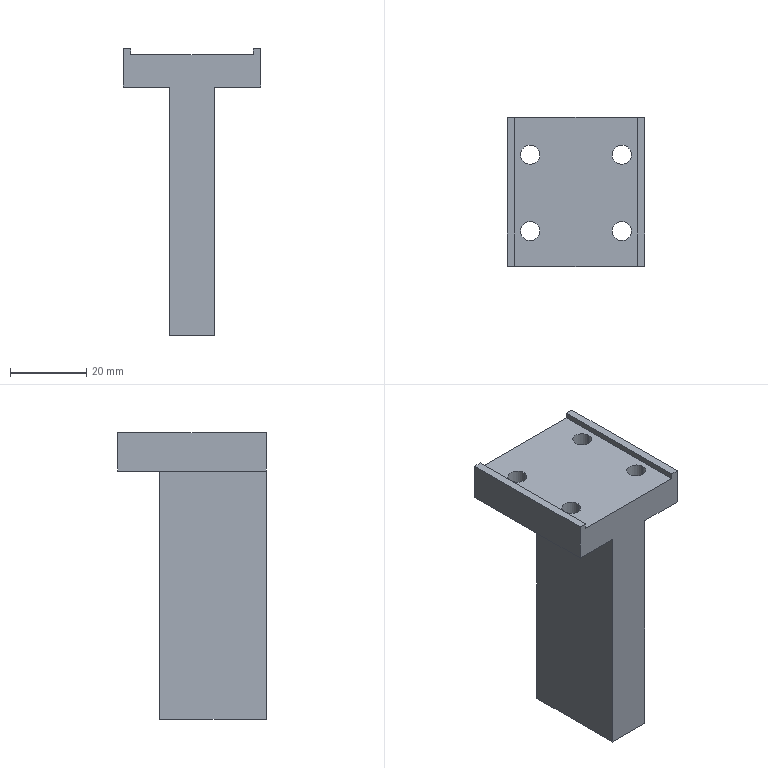Part | SolidWorks | features ICE 4, Extrusion 1, HoleWzd 1 | 1 solid | 22 faces | box 36 x 39 x 75 mm | volume 33340 mm3 | plane 14 | cylinder 8 | commonest cylinder face diameters 5 x8
STEP:
#1=CARTESIAN_POINT('',(14.5,9.7,8.5));
#2=VERTEX_POINT('',#1);
#3=CARTESIAN_POINT('',(9.5,9.7,8.5));
#4=VERTEX_POINT('',#3);
#5=CARTESIAN_POINT('',(12.,9.7,8.5));
#6=DIRECTION('',(0.,0.,-1.));
#7=DIRECTION('',(-1.,0.,0.));
#8=AXIS2_PLACEMENT_3D('',#5,#6,#7);
#9=CIRCLE('',#8,2.5);
#10=EDGE_CURVE('',#2,#4,#9,.T.);
#11=ORIENTED_EDGE('',*,*,#10,.F.);
#12=CARTESIAN_POINT('',(14.5,9.7,0.));
#13=VERTEX_POINT('',#12);
#14=CARTESIAN_POINT('',(14.5,9.7,0.));
#15=DIRECTION('',(0.,0.,-1.));
#16=VECTOR('',#15,1000.);
#17=LINE('',#14,#16);
#18=EDGE_CURVE('',#2,#13,#17,.T.);
#19=ORIENTED_EDGE('',*,*,#18,.T.);
#20=CARTESIAN_POINT('',(9.5,9.7,0.));
#21=VERTEX_POINT('',#20);
#22=CARTESIAN_POINT('',(12.,9.7,0.));
#23=DIRECTION('',(0.,0.,-1.));
#24=DIRECTION('',(-1.,0.,0.));
#25=AXIS2_PLACEMENT_3D('',#22,#23,#24);
#26=CIRCLE('',#25,2.5);
#27=EDGE_CURVE('',#13,#21,#26,.T.);
#28=ORIENTED_EDGE('',*,*,#27,.T.);
#29=CARTESIAN_POINT('',(9.5,9.7,0.));
#30=DIRECTION('',(0.,0.,-1.));
#31=VECTOR('',#30,1000.);
#32=LINE('',#29,#31);
#33=EDGE_CURVE('',#4,#21,#32,.T.);
#34=ORIENTED_EDGE('',*,*,#33,.F.);
#35=EDGE_LOOP('',(#11,#19,#28,#34));
#36=FACE_OUTER_BOUND('',#35,.T.);
#37=CARTESIAN_POINT('',(12.,9.7,0.));
#38=DIRECTION('',(0.,0.,-1.));
#39=DIRECTION('',(-1.,0.,0.));
#40=AXIS2_PLACEMENT_3D('',#37,#38,#39);
#41=CYLINDRICAL_SURFACE('',#40,2.5);
#42=ADVANCED_FACE('',(#36),#41,.F.);
#43=CARTESIAN_POINT('',(-9.5,9.7,8.5));
#44=VERTEX_POINT('',#43);
#45=CARTESIAN_POINT('',(-14.5,9.7,8.5));
#46=VERTEX_POINT('',#45);
#47=CARTESIAN_POINT('',(-12.,9.7,8.5));
#48=DIRECTION('',(0.,0.,-1.));
#49=DIRECTION('',(-1.,0.,0.));
#50=AXIS2_PLACEMENT_3D('',#47,#48,#49);
#51=CIRCLE('',#50,2.5);
#52=EDGE_CURVE('',#44,#46,#51,.T.);
#53=ORIENTED_EDGE('',*,*,#52,.F.);
#54=CARTESIAN_POINT('',(-9.5,9.7,0.));
#55=VERTEX_POINT('',#54);
#56=CARTESIAN_POINT('',(-9.5,9.7,0.));
#57=DIRECTION('',(0.,0.,-1.));
#58=VECTOR('',#57,1000.);
#59=LINE('',#56,#58);
#60=EDGE_CURVE('',#44,#55,#59,.T.);
#61=ORIENTED_EDGE('',*,*,#60,.T.);
#62=CARTESIAN_POINT('',(-14.5,9.7,0.));
#63=VERTEX_POINT('',#62);
#64=CARTESIAN_POINT('',(-12.,9.7,0.));
#65=DIRECTION('',(0.,0.,-1.));
#66=DIRECTION('',(-1.,0.,0.));
#67=AXIS2_PLACEMENT_3D('',#64,#65,#66);
#68=CIRCLE('',#67,2.5);
#69=EDGE_CURVE('',#55,#63,#68,.T.);
#70=ORIENTED_EDGE('',*,*,#69,.T.);
#71=CARTESIAN_POINT('',(-14.5,9.7,0.));
#72=DIRECTION('',(0.,0.,-1.));
#73=VECTOR('',#72,1000.);
#74=LINE('',#71,#73);
#75=EDGE_CURVE('',#46,#63,#74,.T.);
#76=ORIENTED_EDGE('',*,*,#75,.F.);
#77=EDGE_LOOP('',(#53,#61,#70,#76));
#78=FACE_OUTER_BOUND('',#77,.T.);
#79=CARTESIAN_POINT('',(-12.,9.7,0.));
#80=DIRECTION('',(0.,0.,-1.));
#81=DIRECTION('',(-1.,0.,0.));
#82=AXIS2_PLACEMENT_3D('',#79,#80,#81);
#83=CYLINDRICAL_SURFACE('',#82,2.5);
#84=ADVANCED_FACE('',(#78),#83,.F.);
#85=CARTESIAN_POINT('',(-9.5,-10.3,8.5));
#86=VERTEX_POINT('',#85);
#87=CARTESIAN_POINT('',(-14.5,-10.3,8.5));
#88=VERTEX_POINT('',#87);
#89=CARTESIAN_POINT('',(-12.,-10.3,8.5));
#90=DIRECTION('',(0.,0.,-1.));
#91=DIRECTION('',(-1.,0.,0.));
#92=AXIS2_PLACEMENT_3D('',#89,#90,#91);
#93=CIRCLE('',#92,2.5);
#94=EDGE_CURVE('',#86,#88,#93,.T.);
#95=ORIENTED_EDGE('',*,*,#94,.F.);
#96=CARTESIAN_POINT('',(-9.5,-10.3,0.));
#97=VERTEX_POINT('',#96);
#98=CARTESIAN_POINT('',(-9.5,-10.3,0.));
#99=DIRECTION('',(0.,0.,-1.));
#100=VECTOR('',#99,1000.);
#101=LINE('',#98,#100);
#102=EDGE_CURVE('',#86,#97,#101,.T.);
#103=ORIENTED_EDGE('',*,*,#102,.T.);
#104=CARTESIAN_POINT('',(-14.5,-10.3,0.));
#105=VERTEX_POINT('',#104);
#106=CARTESIAN_POINT('',(-12.,-10.3,0.));
#107=DIRECTION('',(0.,0.,-1.));
#108=DIRECTION('',(-1.,0.,0.));
#109=AXIS2_PLACEMENT_3D('',#106,#107,#108);
#110=CIRCLE('',#109,2.5);
#111=EDGE_CURVE('',#97,#105,#110,.T.);
#112=ORIENTED_EDGE('',*,*,#111,.T.);
#113=CARTESIAN_POINT('',(-14.5,-10.3,0.));
#114=DIRECTION('',(0.,0.,-1.));
#115=VECTOR('',#114,1000.);
#116=LINE('',#113,#115);
#117=EDGE_CURVE('',#88,#105,#116,.T.);
#118=ORIENTED_EDGE('',*,*,#117,.F.);
#119=EDGE_LOOP('',(#95,#103,#112,#118));
#120=FACE_OUTER_BOUND('',#119,.T.);
#121=CARTESIAN_POINT('',(-12.,-10.3,0.));
#122=DIRECTION('',(0.,0.,-1.));
#123=DIRECTION('',(-1.,0.,0.));
#124=AXIS2_PLACEMENT_3D('',#121,#122,#123);
#125=CYLINDRICAL_SURFACE('',#124,2.5);
#126=ADVANCED_FACE('',(#120),#125,.F.);
#127=CARTESIAN_POINT('',(14.5,-10.3,8.5));
#128=VERTEX_POINT('',#127);
#129=CARTESIAN_POINT('',(9.5,-10.3,8.5));
#130=VERTEX_POINT('',#129);
#131=CARTESIAN_POINT('',(12.,-10.3,8.5));
#132=DIRECTION('',(0.,0.,-1.));
#133=DIRECTION('',(-1.,0.,0.));
#134=AXIS2_PLACEMENT_3D('',#131,#132,#133);
#135=CIRCLE('',#134,2.5);
#136=EDGE_CURVE('',#128,#130,#135,.T.);
#137=ORIENTED_EDGE('',*,*,#136,.F.);
#138=CARTESIAN_POINT('',(14.5,-10.3,0.));
#139=VERTEX_POINT('',#138);
#140=CARTESIAN_POINT('',(14.5,-10.3,0.));
#141=DIRECTION('',(0.,0.,-1.));
#142=VECTOR('',#141,1000.);
#143=LINE('',#140,#142);
#144=EDGE_CURVE('',#128,#139,#143,.T.);
#145=ORIENTED_EDGE('',*,*,#144,.T.);
#146=CARTESIAN_POINT('',(9.5,-10.3,0.));
#147=VERTEX_POINT('',#146);
#148=CARTESIAN_POINT('',(12.,-10.3,0.));
#149=DIRECTION('',(0.,0.,-1.));
#150=DIRECTION('',(-1.,0.,0.));
#151=AXIS2_PLACEMENT_3D('',#148,#149,#150);
#152=CIRCLE('',#151,2.5);
#153=EDGE_CURVE('',#139,#147,#152,.T.);
#154=ORIENTED_EDGE('',*,*,#153,.T.);
#155=CARTESIAN_POINT('',(9.5,-10.3,0.));
#156=DIRECTION('',(0.,0.,-1.));
#157=VECTOR('',#156,1000.);
#158=LINE('',#155,#157);
#159=EDGE_CURVE('',#130,#147,#158,.T.);
#160=ORIENTED_EDGE('',*,*,#159,.F.);
#161=EDGE_LOOP('',(#137,#145,#154,#160));
#162=FACE_OUTER_BOUND('',#161,.T.);
#163=CARTESIAN_POINT('',(12.,-10.3,0.));
#164=DIRECTION('',(0.,0.,-1.));
#165=DIRECTION('',(-1.,0.,0.));
#166=AXIS2_PLACEMENT_3D('',#163,#164,#165);
#167=CYLINDRICAL_SURFACE('',#166,2.5);
#168=ADVANCED_FACE('',(#162),#167,.F.);
#169=CARTESIAN_POINT('',(18.,19.5,10.));
#170=VERTEX_POINT('',#169);
#171=CARTESIAN_POINT('',(16.,19.5,10.));
#172=VERTEX_POINT('',#171);
#173=CARTESIAN_POINT('',(-18.,19.5,10.));
#174=DIRECTION('',(-1.,0.,0.));
#175=VECTOR('',#174,1000.);
#176=LINE('',#173,#175);
#177=EDGE_CURVE('',#170,#172,#176,.T.);
#178=ORIENTED_EDGE('',*,*,#177,.T.);
#179=CARTESIAN_POINT('',(16.,-19.5,10.));
#180=VERTEX_POINT('',#179);
#181=CARTESIAN_POINT('',(16.,-19.5,10.));
#182=DIRECTION('',(0.,1.,0.));
#183=VECTOR('',#182,1000.);
#184=LINE('',#181,#183);
#185=EDGE_CURVE('',#180,#172,#184,.T.);
#186=ORIENTED_EDGE('',*,*,#185,.F.);
#187=CARTESIAN_POINT('',(18.,-19.5,10.));
#188=VERTEX_POINT('',#187);
#189=CARTESIAN_POINT('',(-18.,-19.5,10.));
#190=DIRECTION('',(1.,0.,0.));
#191=VECTOR('',#190,1000.);
#192=LINE('',#189,#191);
#193=EDGE_CURVE('',#180,#188,#192,.T.);
#194=ORIENTED_EDGE('',*,*,#193,.T.);
#195=CARTESIAN_POINT('',(18.,-19.5,10.));
#196=DIRECTION('',(0.,1.,0.));
#197=VECTOR('',#196,1000.);
#198=LINE('',#195,#197);
#199=EDGE_CURVE('',#188,#170,#198,.T.);
#200=ORIENTED_EDGE('',*,*,#199,.T.);
#201=EDGE_LOOP('',(#178,#186,#194,#200));
#202=FACE_OUTER_BOUND('',#201,.T.);
#203=CARTESIAN_POINT('',(0.,0.,10.));
#204=DIRECTION('',(0.,0.,-1.));
#205=DIRECTION('',(-1.,0.,0.));
#206=AXIS2_PLACEMENT_3D('',#203,#204,#205);
#207=PLANE('',#206);
#208=ADVANCED_FACE('',(#202),#207,.F.);
#209=CARTESIAN_POINT('',(18.,-19.5,0.));
#210=VERTEX_POINT('',#209);
#211=CARTESIAN_POINT('',(18.,19.5,0.));
#212=VERTEX_POINT('',#211);
#213=CARTESIAN_POINT('',(18.,-19.5,0.));
#214=DIRECTION('',(0.,1.,0.));
#215=VECTOR('',#214,1000.);
#216=LINE('',#213,#215);
#217=EDGE_CURVE('',#210,#212,#216,.T.);
#218=ORIENTED_EDGE('',*,*,#217,.T.);
#219=CARTESIAN_POINT('',(18.,19.5,10.));
#220=DIRECTION('',(0.,0.,-1.));
#221=VECTOR('',#220,1000.);
#222=LINE('',#219,#221);
#223=EDGE_CURVE('',#170,#212,#222,.T.);
#224=ORIENTED_EDGE('',*,*,#223,.F.);
#225=ORIENTED_EDGE('',*,*,#199,.F.);
#226=CARTESIAN_POINT('',(18.,-19.5,10.));
#227=DIRECTION('',(0.,0.,-1.));
#228=VECTOR('',#227,1000.);
#229=LINE('',#226,#228);
#230=EDGE_CURVE('',#188,#210,#229,.T.);
#231=ORIENTED_EDGE('',*,*,#230,.T.);
#232=EDGE_LOOP('',(#218,#224,#225,#231));
#233=FACE_OUTER_BOUND('',#232,.T.);
#234=CARTESIAN_POINT('',(18.,-19.5,10.));
#235=DIRECTION('',(-1.,0.,0.));
#236=DIRECTION('',(0.,0.,1.));
#237=AXIS2_PLACEMENT_3D('',#234,#235,#236);
#238=PLANE('',#237);
#239=ADVANCED_FACE('',(#233),#238,.F.);
#240=CARTESIAN_POINT('',(16.,19.5,8.5));
#241=VERTEX_POINT('',#240);
#242=CARTESIAN_POINT('',(-16.,19.5,8.5));
#243=VERTEX_POINT('',#242);
#244=CARTESIAN_POINT('',(-16.,19.5,8.5));
#245=DIRECTION('',(-1.,0.,0.));
#246=VECTOR('',#245,1000.);
#247=LINE('',#244,#246);
#248=EDGE_CURVE('',#241,#243,#247,.T.);
#249=ORIENTED_EDGE('',*,*,#248,.F.);
#250=CARTESIAN_POINT('',(16.,19.5,8.5));
#251=DIRECTION('',(0.,0.,1.));
#252=VECTOR('',#251,1000.);
#253=LINE('',#250,#252);
#254=EDGE_CURVE('',#241,#172,#253,.T.);
#255=ORIENTED_EDGE('',*,*,#254,.T.);
#256=ORIENTED_EDGE('',*,*,#177,.F.);
#257=ORIENTED_EDGE('',*,*,#223,.T.);
#258=CARTESIAN_POINT('',(-18.,19.5,0.));
#259=VERTEX_POINT('',#258);
#260=CARTESIAN_POINT('',(-18.,19.5,0.));
#261=DIRECTION('',(-1.,0.,0.));
#262=VECTOR('',#261,1000.);
#263=LINE('',#260,#262);
#264=EDGE_CURVE('',#212,#259,#263,.T.);
#265=ORIENTED_EDGE('',*,*,#264,.T.);
#266=CARTESIAN_POINT('',(-18.,19.5,10.));
#267=VERTEX_POINT('',#266);
#268=CARTESIAN_POINT('',(-18.,19.5,10.));
#269=DIRECTION('',(0.,0.,-1.));
#270=VECTOR('',#269,1000.);
#271=LINE('',#268,#270);
#272=EDGE_CURVE('',#267,#259,#271,.T.);
#273=ORIENTED_EDGE('',*,*,#272,.F.);
#274=CARTESIAN_POINT('',(-16.,19.5,10.));
#275=VERTEX_POINT('',#274);
#276=CARTESIAN_POINT('',(-18.,19.5,10.));
#277=DIRECTION('',(-1.,0.,0.));
#278=VECTOR('',#277,1000.);
#279=LINE('',#276,#278);
#280=EDGE_CURVE('',#275,#267,#279,.T.);
#281=ORIENTED_EDGE('',*,*,#280,.F.);
#282=CARTESIAN_POINT('',(-16.,19.5,8.5));
#283=DIRECTION('',(0.,0.,1.));
#284=VECTOR('',#283,1000.);
#285=LINE('',#282,#284);
#286=EDGE_CURVE('',#243,#275,#285,.T.);
#287=ORIENTED_EDGE('',*,*,#286,.F.);
#288=EDGE_LOOP('',(#249,#255,#256,#257,#265,#273,#281,#287));
#289=FACE_OUTER_BOUND('',#288,.T.);
#290=CARTESIAN_POINT('',(-18.,19.5,10.));
#291=DIRECTION('',(0.,-1.,0.));
#292=DIRECTION('',(0.,0.,-1.));
#293=AXIS2_PLACEMENT_3D('',#290,#291,#292);
#294=PLANE('',#293);
#295=ADVANCED_FACE('',(#289),#294,.F.);
#296=CARTESIAN_POINT('',(-18.,-19.5,0.));
#297=VERTEX_POINT('',#296);
#298=CARTESIAN_POINT('',(-18.,-19.5,0.));
#299=DIRECTION('',(0.,-1.,0.));
#300=VECTOR('',#299,1000.);
#301=LINE('',#298,#300);
#302=EDGE_CURVE('',#259,#297,#301,.T.);
#303=ORIENTED_EDGE('',*,*,#302,.T.);
#304=CARTESIAN_POINT('',(-18.,-19.5,10.));
#305=VERTEX_POINT('',#304);
#306=CARTESIAN_POINT('',(-18.,-19.5,10.));
#307=DIRECTION('',(0.,0.,-1.));
#308=VECTOR('',#307,1000.);
#309=LINE('',#306,#308);
#310=EDGE_CURVE('',#305,#297,#309,.T.);
#311=ORIENTED_EDGE('',*,*,#310,.F.);
#312=CARTESIAN_POINT('',(-18.,-19.5,10.));
#313=DIRECTION('',(0.,-1.,0.));
#314=VECTOR('',#313,1000.);
#315=LINE('',#312,#314);
#316=EDGE_CURVE('',#267,#305,#315,.T.);
#317=ORIENTED_EDGE('',*,*,#316,.F.);
#318=ORIENTED_EDGE('',*,*,#272,.T.);
#319=EDGE_LOOP('',(#303,#311,#317,#318));
#320=FACE_OUTER_BOUND('',#319,.T.);
#321=CARTESIAN_POINT('',(-18.,-19.5,10.));
#322=DIRECTION('',(1.,0.,0.));
#323=DIRECTION('',(0.,0.,-1.));
#324=AXIS2_PLACEMENT_3D('',#321,#322,#323);
#325=PLANE('',#324);
#326=ADVANCED_FACE('',(#320),#325,.F.);
#327=ORIENTED_EDGE('',*,*,#193,.F.);
#328=CARTESIAN_POINT('',(16.,-19.5,8.5));
#329=VERTEX_POINT('',#328);
#330=CARTESIAN_POINT('',(16.,-19.5,8.5));
#331=DIRECTION('',(0.,0.,1.));
#332=VECTOR('',#331,1000.);
#333=LINE('',#330,#332);
#334=EDGE_CURVE('',#329,#180,#333,.T.);
#335=ORIENTED_EDGE('',*,*,#334,.F.);
#336=CARTESIAN_POINT('',(-16.,-19.5,8.5));
#337=VERTEX_POINT('',#336);
#338=CARTESIAN_POINT('',(-16.,-19.5,8.5));
#339=DIRECTION('',(1.,0.,0.));
#340=VECTOR('',#339,1000.);
#341=LINE('',#338,#340);
#342=EDGE_CURVE('',#337,#329,#341,.T.);
#343=ORIENTED_EDGE('',*,*,#342,.F.);
#344=CARTESIAN_POINT('',(-16.,-19.5,10.));
#345=VERTEX_POINT('',#344);
#346=CARTESIAN_POINT('',(-16.,-19.5,8.5));
#347=DIRECTION('',(0.,0.,1.));
#348=VECTOR('',#347,1000.);
#349=LINE('',#346,#348);
#350=EDGE_CURVE('',#337,#345,#349,.T.);
#351=ORIENTED_EDGE('',*,*,#350,.T.);
#352=CARTESIAN_POINT('',(-18.,-19.5,10.));
#353=DIRECTION('',(1.,0.,0.));
#354=VECTOR('',#353,1000.);
#355=LINE('',#352,#354);
#356=EDGE_CURVE('',#305,#345,#355,.T.);
#357=ORIENTED_EDGE('',*,*,#356,.F.);
#358=ORIENTED_EDGE('',*,*,#310,.T.);
#359=CARTESIAN_POINT('',(-6.,-19.5,0.));
#360=VERTEX_POINT('',#359);
#361=CARTESIAN_POINT('',(-18.,-19.5,0.));
#362=DIRECTION('',(1.,0.,0.));
#363=VECTOR('',#362,1000.);
#364=LINE('',#361,#363);
#365=EDGE_CURVE('',#297,#360,#364,.T.);
#366=ORIENTED_EDGE('',*,*,#365,.T.);
#367=CARTESIAN_POINT('',(-6.,-19.5,-65.));
#368=VERTEX_POINT('',#367);
#369=CARTESIAN_POINT('',(-6.,-19.5,-65.));
#370=DIRECTION('',(0.,0.,1.));
#371=VECTOR('',#370,1000.);
#372=LINE('',#369,#371);
#373=EDGE_CURVE('',#368,#360,#372,.T.);
#374=ORIENTED_EDGE('',*,*,#373,.F.);
#375=CARTESIAN_POINT('',(6.,-19.5,-65.));
#376=VERTEX_POINT('',#375);
#377=CARTESIAN_POINT('',(6.,-19.5,-65.));
#378=DIRECTION('',(-1.,0.,0.));
#379=VECTOR('',#378,1000.);
#380=LINE('',#377,#379);
#381=EDGE_CURVE('',#376,#368,#380,.T.);
#382=ORIENTED_EDGE('',*,*,#381,.F.);
#383=CARTESIAN_POINT('',(6.,-19.5,0.));
#384=VERTEX_POINT('',#383);
#385=CARTESIAN_POINT('',(6.,-19.5,-65.));
#386=DIRECTION('',(0.,0.,1.));
#387=VECTOR('',#386,1000.);
#388=LINE('',#385,#387);
#389=EDGE_CURVE('',#376,#384,#388,.T.);
#390=ORIENTED_EDGE('',*,*,#389,.T.);
#391=CARTESIAN_POINT('',(-18.,-19.5,0.));
#392=DIRECTION('',(1.,0.,0.));
#393=VECTOR('',#392,1000.);
#394=LINE('',#391,#393);
#395=EDGE_CURVE('',#384,#210,#394,.T.);
#396=ORIENTED_EDGE('',*,*,#395,.T.);
#397=ORIENTED_EDGE('',*,*,#230,.F.);
#398=EDGE_LOOP('',(#327,#335,#343,#351,#357,#358,#366,#374,#382,#390,#396,#397));
#399=FACE_OUTER_BOUND('',#398,.T.);
#400=CARTESIAN_POINT('',(-18.,-19.5,10.));
#401=DIRECTION('',(0.,1.,0.));
#402=DIRECTION('',(0.,0.,1.));
#403=AXIS2_PLACEMENT_3D('',#400,#401,#402);
#404=PLANE('',#403);
#405=ADVANCED_FACE('',(#399),#404,.F.);
#406=ORIENTED_EDGE('',*,*,#356,.T.);
#407=CARTESIAN_POINT('',(-16.,-19.5,10.));
#408=DIRECTION('',(0.,-1.,0.));
#409=VECTOR('',#408,1000.);
#410=LINE('',#407,#409);
#411=EDGE_CURVE('',#275,#345,#410,.T.);
#412=ORIENTED_EDGE('',*,*,#411,.F.);
#413=ORIENTED_EDGE('',*,*,#280,.T.);
#414=ORIENTED_EDGE('',*,*,#316,.T.);
#415=EDGE_LOOP('',(#406,#412,#413,#414));
#416=FACE_OUTER_BOUND('',#415,.T.);
#417=CARTESIAN_POINT('',(0.,0.,10.));
#418=DIRECTION('',(0.,0.,-1.));
#419=DIRECTION('',(-1.,0.,0.));
#420=AXIS2_PLACEMENT_3D('',#417,#418,#419);
#421=PLANE('',#420);
#422=ADVANCED_FACE('',(#416),#421,.F.);
#423=CARTESIAN_POINT('',(12.,9.7,0.));
#424=DIRECTION('',(0.,0.,-1.));
#425=DIRECTION('',(-1.,0.,0.));
#426=AXIS2_PLACEMENT_3D('',#423,#424,#425);
#427=CIRCLE('',#426,2.5);
#428=EDGE_CURVE('',#21,#13,#427,.T.);
#429=ORIENTED_EDGE('',*,*,#428,.F.);
#430=ORIENTED_EDGE('',*,*,#27,.F.);
#431=EDGE_LOOP('',(#429,#430));
#432=FACE_BOUND('',#431,.T.);
#433=CARTESIAN_POINT('',(-12.,9.7,0.));
#434=DIRECTION('',(0.,0.,-1.));
#435=DIRECTION('',(-1.,0.,0.));
#436=AXIS2_PLACEMENT_3D('',#433,#434,#435);
#437=CIRCLE('',#436,2.5);
#438=EDGE_CURVE('',#63,#55,#437,.T.);
#439=ORIENTED_EDGE('',*,*,#438,.F.);
#440=ORIENTED_EDGE('',*,*,#69,.F.);
#441=EDGE_LOOP('',(#439,#440));
#442=FACE_BOUND('',#441,.T.);
#443=CARTESIAN_POINT('',(-12.,-10.3,0.));
#444=DIRECTION('',(0.,0.,-1.));
#445=DIRECTION('',(-1.,0.,0.));
#446=AXIS2_PLACEMENT_3D('',#443,#444,#445);
#447=CIRCLE('',#446,2.5);
#448=EDGE_CURVE('',#105,#97,#447,.T.);
#449=ORIENTED_EDGE('',*,*,#448,.F.);
#450=ORIENTED_EDGE('',*,*,#111,.F.);
#451=EDGE_LOOP('',(#449,#450));
#452=FACE_BOUND('',#451,.T.);
#453=CARTESIAN_POINT('',(12.,-10.3,0.));
#454=DIRECTION('',(0.,0.,-1.));
#455=DIRECTION('',(-1.,0.,0.));
#456=AXIS2_PLACEMENT_3D('',#453,#454,#455);
#457=CIRCLE('',#456,2.5);
#458=EDGE_CURVE('',#147,#139,#457,.T.);
#459=ORIENTED_EDGE('',*,*,#458,.F.);
#460=ORIENTED_EDGE('',*,*,#153,.F.);
#461=EDGE_LOOP('',(#459,#460));
#462=FACE_BOUND('',#461,.T.);
#463=CARTESIAN_POINT('',(6.,8.5,0.));
#464=VERTEX_POINT('',#463);
#465=CARTESIAN_POINT('',(6.,-19.5,0.));
#466=DIRECTION('',(0.,-1.,0.));
#467=VECTOR('',#466,1000.);
#468=LINE('',#465,#467);
#469=EDGE_CURVE('',#464,#384,#468,.T.);
#470=ORIENTED_EDGE('',*,*,#469,.F.);
#471=CARTESIAN_POINT('',(-6.,8.5,0.));
#472=VERTEX_POINT('',#471);
#473=CARTESIAN_POINT('',(6.,8.5,0.));
#474=DIRECTION('',(1.,0.,0.));
#475=VECTOR('',#474,1000.);
#476=LINE('',#473,#475);
#477=EDGE_CURVE('',#472,#464,#476,.T.);
#478=ORIENTED_EDGE('',*,*,#477,.F.);
#479=CARTESIAN_POINT('',(-6.,-19.5,0.));
#480=DIRECTION('',(0.,1.,0.));
#481=VECTOR('',#480,1000.);
#482=LINE('',#479,#481);
#483=EDGE_CURVE('',#360,#472,#482,.T.);
#484=ORIENTED_EDGE('',*,*,#483,.F.);
#485=ORIENTED_EDGE('',*,*,#365,.F.);
#486=ORIENTED_EDGE('',*,*,#302,.F.);
#487=ORIENTED_EDGE('',*,*,#264,.F.);
#488=ORIENTED_EDGE('',*,*,#217,.F.);
#489=ORIENTED_EDGE('',*,*,#395,.F.);
#490=EDGE_LOOP('',(#470,#478,#484,#485,#486,#487,#488,#489));
#491=FACE_OUTER_BOUND('',#490,.T.);
#492=CARTESIAN_POINT('',(0.,0.,0.));
#493=DIRECTION('',(0.,0.,-1.));
#494=DIRECTION('',(-1.,0.,0.));
#495=AXIS2_PLACEMENT_3D('',#492,#493,#494);
#496=PLANE('',#495);
#497=ADVANCED_FACE('',(#432,#442,#452,#462,#491),#496,.T.);
#498=ORIENTED_EDGE('',*,*,#185,.T.);
#499=ORIENTED_EDGE('',*,*,#254,.F.);
#500=CARTESIAN_POINT('',(16.,-19.5,8.5));
#501=DIRECTION('',(0.,1.,0.));
#502=VECTOR('',#501,1000.);
#503=LINE('',#500,#502);
#504=EDGE_CURVE('',#329,#241,#503,.T.);
#505=ORIENTED_EDGE('',*,*,#504,.F.);
#506=ORIENTED_EDGE('',*,*,#334,.T.);
#507=EDGE_LOOP('',(#498,#499,#505,#506));
#508=FACE_OUTER_BOUND('',#507,.T.);
#509=CARTESIAN_POINT('',(16.,-19.5,8.5));
#510=DIRECTION('',(1.,0.,0.));
#511=DIRECTION('',(0.,0.,-1.));
#512=AXIS2_PLACEMENT_3D('',#509,#510,#511);
#513=PLANE('',#512);
#514=ADVANCED_FACE('',(#508),#513,.F.);
#515=ORIENTED_EDGE('',*,*,#411,.T.);
#516=ORIENTED_EDGE('',*,*,#350,.F.);
#517=CARTESIAN_POINT('',(-16.,-19.5,8.5));
#518=DIRECTION('',(0.,-1.,0.));
#519=VECTOR('',#518,1000.);
#520=LINE('',#517,#519);
#521=EDGE_CURVE('',#243,#337,#520,.T.);
#522=ORIENTED_EDGE('',*,*,#521,.F.);
#523=ORIENTED_EDGE('',*,*,#286,.T.);
#524=EDGE_LOOP('',(#515,#516,#522,#523));
#525=FACE_OUTER_BOUND('',#524,.T.);
#526=CARTESIAN_POINT('',(-16.,-19.5,8.5));
#527=DIRECTION('',(-1.,0.,0.));
#528=DIRECTION('',(0.,0.,1.));
#529=AXIS2_PLACEMENT_3D('',#526,#527,#528);
#530=PLANE('',#529);
#531=ADVANCED_FACE('',(#525),#530,.F.);
#532=CARTESIAN_POINT('',(12.,9.7,8.5));
#533=DIRECTION('',(0.,0.,-1.));
#534=DIRECTION('',(-1.,0.,0.));
#535=AXIS2_PLACEMENT_3D('',#532,#533,#534);
#536=CIRCLE('',#535,2.5);
#537=EDGE_CURVE('',#4,#2,#536,.T.);
#538=ORIENTED_EDGE('',*,*,#537,.T.);
#539=ORIENTED_EDGE('',*,*,#10,.T.);
#540=EDGE_LOOP('',(#538,#539));
#541=FACE_BOUND('',#540,.T.);
#542=CARTESIAN_POINT('',(-12.,9.7,8.5));
#543=DIRECTION('',(0.,0.,-1.));
#544=DIRECTION('',(-1.,0.,0.));
#545=AXIS2_PLACEMENT_3D('',#542,#543,#544);
#546=CIRCLE('',#545,2.5);
#547=EDGE_CURVE('',#46,#44,#546,.T.);
#548=ORIENTED_EDGE('',*,*,#547,.T.);
#549=ORIENTED_EDGE('',*,*,#52,.T.);
#550=EDGE_LOOP('',(#548,#549));
#551=FACE_BOUND('',#550,.T.);
#552=CARTESIAN_POINT('',(-12.,-10.3,8.5));
#553=DIRECTION('',(0.,0.,-1.));
#554=DIRECTION('',(-1.,0.,0.));
#555=AXIS2_PLACEMENT_3D('',#552,#553,#554);
#556=CIRCLE('',#555,2.5);
#557=EDGE_CURVE('',#88,#86,#556,.T.);
#558=ORIENTED_EDGE('',*,*,#557,.T.);
#559=ORIENTED_EDGE('',*,*,#94,.T.);
#560=EDGE_LOOP('',(#558,#559));
#561=FACE_BOUND('',#560,.T.);
#562=CARTESIAN_POINT('',(12.,-10.3,8.5));
#563=DIRECTION('',(0.,0.,-1.));
#564=DIRECTION('',(-1.,0.,0.));
#565=AXIS2_PLACEMENT_3D('',#562,#563,#564);
#566=CIRCLE('',#565,2.5);
#567=EDGE_CURVE('',#130,#128,#566,.T.);
#568=ORIENTED_EDGE('',*,*,#567,.T.);
#569=ORIENTED_EDGE('',*,*,#136,.T.);
#570=EDGE_LOOP('',(#568,#569));
#571=FACE_BOUND('',#570,.T.);
#572=ORIENTED_EDGE('',*,*,#504,.T.);
#573=ORIENTED_EDGE('',*,*,#248,.T.);
#574=ORIENTED_EDGE('',*,*,#521,.T.);
#575=ORIENTED_EDGE('',*,*,#342,.T.);
#576=EDGE_LOOP('',(#572,#573,#574,#575));
#577=FACE_OUTER_BOUND('',#576,.T.);
#578=CARTESIAN_POINT('',(0.,0.,8.5));
#579=DIRECTION('',(0.,0.,-1.));
#580=DIRECTION('',(-1.,0.,0.));
#581=AXIS2_PLACEMENT_3D('',#578,#579,#580);
#582=PLANE('',#581);
#583=ADVANCED_FACE('',(#541,#551,#561,#571,#577),#582,.F.);
#584=ORIENTED_EDGE('',*,*,#469,.T.);
#585=ORIENTED_EDGE('',*,*,#389,.F.);
#586=CARTESIAN_POINT('',(6.,8.5,-65.));
#587=VERTEX_POINT('',#586);
#588=CARTESIAN_POINT('',(6.,-19.5,-65.));
#589=DIRECTION('',(0.,-1.,0.));
#590=VECTOR('',#589,1000.);
#591=LINE('',#588,#590);
#592=EDGE_CURVE('',#587,#376,#591,.T.);
#593=ORIENTED_EDGE('',*,*,#592,.F.);
#594=CARTESIAN_POINT('',(6.,8.5,-65.));
#595=DIRECTION('',(0.,0.,1.));
#596=VECTOR('',#595,1000.);
#597=LINE('',#594,#596);
#598=EDGE_CURVE('',#587,#464,#597,.T.);
#599=ORIENTED_EDGE('',*,*,#598,.T.);
#600=EDGE_LOOP('',(#584,#585,#593,#599));
#601=FACE_OUTER_BOUND('',#600,.T.);
#602=CARTESIAN_POINT('',(6.,-19.5,-65.));
#603=DIRECTION('',(-1.,0.,0.));
#604=DIRECTION('',(0.,0.,1.));
#605=AXIS2_PLACEMENT_3D('',#602,#603,#604);
#606=PLANE('',#605);
#607=ADVANCED_FACE('',(#601),#606,.F.);
#608=ORIENTED_EDGE('',*,*,#483,.T.);
#609=CARTESIAN_POINT('',(-6.,8.5,-65.));
#610=VERTEX_POINT('',#609);
#611=CARTESIAN_POINT('',(-6.,8.5,-65.));
#612=DIRECTION('',(0.,0.,1.));
#613=VECTOR('',#612,1000.);
#614=LINE('',#611,#613);
#615=EDGE_CURVE('',#610,#472,#614,.T.);
#616=ORIENTED_EDGE('',*,*,#615,.F.);
#617=CARTESIAN_POINT('',(-6.,-19.5,-65.));
#618=DIRECTION('',(0.,1.,0.));
#619=VECTOR('',#618,1000.);
#620=LINE('',#617,#619);
#621=EDGE_CURVE('',#368,#610,#620,.T.);
#622=ORIENTED_EDGE('',*,*,#621,.F.);
#623=ORIENTED_EDGE('',*,*,#373,.T.);
#624=EDGE_LOOP('',(#608,#616,#622,#623));
#625=FACE_OUTER_BOUND('',#624,.T.);
#626=CARTESIAN_POINT('',(-6.,-19.5,-65.));
#627=DIRECTION('',(1.,0.,0.));
#628=DIRECTION('',(0.,0.,-1.));
#629=AXIS2_PLACEMENT_3D('',#626,#627,#628);
#630=PLANE('',#629);
#631=ADVANCED_FACE('',(#625),#630,.F.);
#632=ORIENTED_EDGE('',*,*,#477,.T.);
#633=ORIENTED_EDGE('',*,*,#598,.F.);
#634=CARTESIAN_POINT('',(6.,8.5,-65.));
#635=DIRECTION('',(1.,0.,0.));
#636=VECTOR('',#635,1000.);
#637=LINE('',#634,#636);
#638=EDGE_CURVE('',#610,#587,#637,.T.);
#639=ORIENTED_EDGE('',*,*,#638,.F.);
#640=ORIENTED_EDGE('',*,*,#615,.T.);
#641=EDGE_LOOP('',(#632,#633,#639,#640));
#642=FACE_OUTER_BOUND('',#641,.T.);
#643=CARTESIAN_POINT('',(6.,8.5,-65.));
#644=DIRECTION('',(0.,-1.,0.));
#645=DIRECTION('',(0.,0.,-1.));
#646=AXIS2_PLACEMENT_3D('',#643,#644,#645);
#647=PLANE('',#646);
#648=ADVANCED_FACE('',(#642),#647,.F.);
#649=ORIENTED_EDGE('',*,*,#592,.T.);
#650=ORIENTED_EDGE('',*,*,#381,.T.);
#651=ORIENTED_EDGE('',*,*,#621,.T.);
#652=ORIENTED_EDGE('',*,*,#638,.T.);
#653=EDGE_LOOP('',(#649,#650,#651,#652));
#654=FACE_OUTER_BOUND('',#653,.T.);
#655=CARTESIAN_POINT('',(0.,0.,-65.));
#656=DIRECTION('',(0.,0.,1.));
#657=DIRECTION('',(1.,0.,0.));
#658=AXIS2_PLACEMENT_3D('',#655,#656,#657);
#659=PLANE('',#658);
#660=ADVANCED_FACE('',(#654),#659,.F.);
#661=ORIENTED_EDGE('',*,*,#144,.F.);
#662=ORIENTED_EDGE('',*,*,#567,.F.);
#663=ORIENTED_EDGE('',*,*,#159,.T.);
#664=ORIENTED_EDGE('',*,*,#458,.T.);
#665=EDGE_LOOP('',(#661,#662,#663,#664));
#666=FACE_OUTER_BOUND('',#665,.T.);
#667=CARTESIAN_POINT('',(12.,-10.3,0.));
#668=DIRECTION('',(0.,0.,-1.));
#669=DIRECTION('',(-1.,0.,0.));
#670=AXIS2_PLACEMENT_3D('',#667,#668,#669);
#671=CYLINDRICAL_SURFACE('',#670,2.5);
#672=ADVANCED_FACE('',(#666),#671,.F.);
#673=ORIENTED_EDGE('',*,*,#102,.F.);
#674=ORIENTED_EDGE('',*,*,#557,.F.);
#675=ORIENTED_EDGE('',*,*,#117,.T.);
#676=ORIENTED_EDGE('',*,*,#448,.T.);
#677=EDGE_LOOP('',(#673,#674,#675,#676));
#678=FACE_OUTER_BOUND('',#677,.T.);
#679=CARTESIAN_POINT('',(-12.,-10.3,0.));
#680=DIRECTION('',(0.,0.,-1.));
#681=DIRECTION('',(-1.,0.,0.));
#682=AXIS2_PLACEMENT_3D('',#679,#680,#681);
#683=CYLINDRICAL_SURFACE('',#682,2.5);
#684=ADVANCED_FACE('',(#678),#683,.F.);
#685=ORIENTED_EDGE('',*,*,#60,.F.);
#686=ORIENTED_EDGE('',*,*,#547,.F.);
#687=ORIENTED_EDGE('',*,*,#75,.T.);
#688=ORIENTED_EDGE('',*,*,#438,.T.);
#689=EDGE_LOOP('',(#685,#686,#687,#688));
#690=FACE_OUTER_BOUND('',#689,.T.);
#691=CARTESIAN_POINT('',(-12.,9.7,0.));
#692=DIRECTION('',(0.,0.,-1.));
#693=DIRECTION('',(-1.,0.,0.));
#694=AXIS2_PLACEMENT_3D('',#691,#692,#693);
#695=CYLINDRICAL_SURFACE('',#694,2.5);
#696=ADVANCED_FACE('',(#690),#695,.F.);
#697=ORIENTED_EDGE('',*,*,#18,.F.);
#698=ORIENTED_EDGE('',*,*,#537,.F.);
#699=ORIENTED_EDGE('',*,*,#33,.T.);
#700=ORIENTED_EDGE('',*,*,#428,.T.);
#701=EDGE_LOOP('',(#697,#698,#699,#700));
#702=FACE_OUTER_BOUND('',#701,.T.);
#703=CARTESIAN_POINT('',(12.,9.7,0.));
#704=DIRECTION('',(0.,0.,-1.));
#705=DIRECTION('',(-1.,0.,0.));
#706=AXIS2_PLACEMENT_3D('',#703,#704,#705);
#707=CYLINDRICAL_SURFACE('',#706,2.5);
#708=ADVANCED_FACE('',(#702),#707,.F.);
#709=CLOSED_SHELL('',(#42,#84,#126,#168,#208,#239,#295,#326,#405,#422,#497,#514,#531,#583,#607,#631,#648,#660,#672,#684,#696,#708));
#710=MANIFOLD_SOLID_BREP('',#709);
#711=CARTESIAN_POINT('',(0.,0.,0.));
#712=DIRECTION('',(0.,0.,1.));
#713=DIRECTION('',(1.,0.,0.));
#714=AXIS2_PLACEMENT_3D('',#711,#712,#713);
#715=(LENGTH_UNIT()NAMED_UNIT(*)SI_UNIT(.MILLI.,.METRE.));
#716=UNCERTAINTY_MEASURE_WITH_UNIT(LENGTH_MEASURE(0.00001),#715,'','');
#717=(NAMED_UNIT(*)PLANE_ANGLE_UNIT()SI_UNIT($,.RADIAN.));
#718=(NAMED_UNIT(*)SI_UNIT($,.STERADIAN.)SOLID_ANGLE_UNIT());
#719=(GEOMETRIC_REPRESENTATION_CONTEXT(3)GLOBAL_UNCERTAINTY_ASSIGNED_CONTEXT((#716))GLOBAL_UNIT_ASSIGNED_CONTEXT((#715,#717,#718))REPRESENTATION_CONTEXT('',''));
#720=ADVANCED_BREP_SHAPE_REPRESENTATION('',(#710,#714),#719);